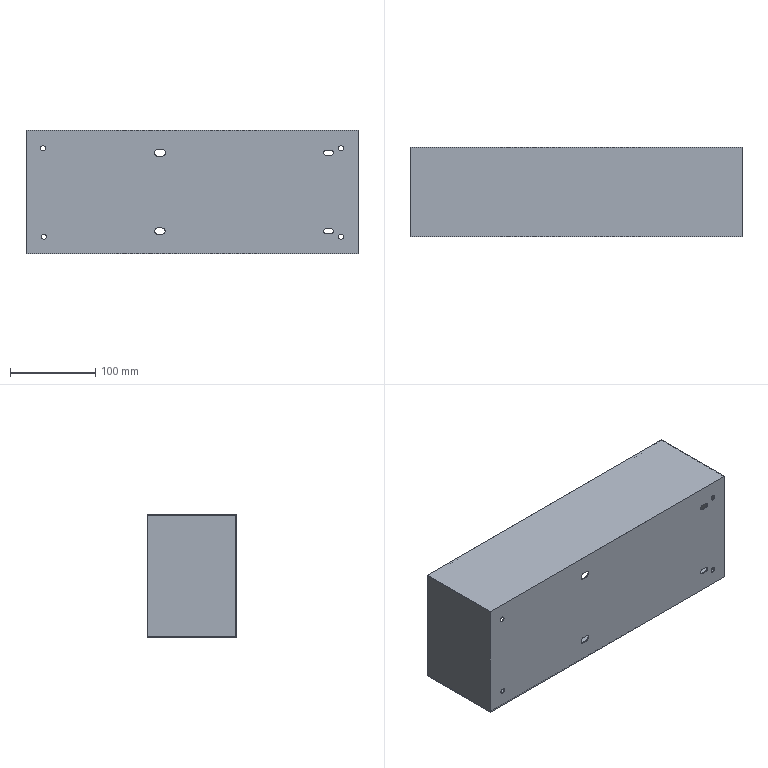Part | SolidWorks | features MoveFace 10, ICE 3, Extrusion 1, Fillet 1, HoleWzd 1, Scale 1, Shell 1 | 1 solid | 63 faces | box 390 x 105 x 144.75 mm | volume 168659 mm3 | cylinder 32 | plane 31 | commonest cylinder face diameters 4.95 x8 6 x8 15 x8 6.4 x4 7.505 x2 7.743 x2